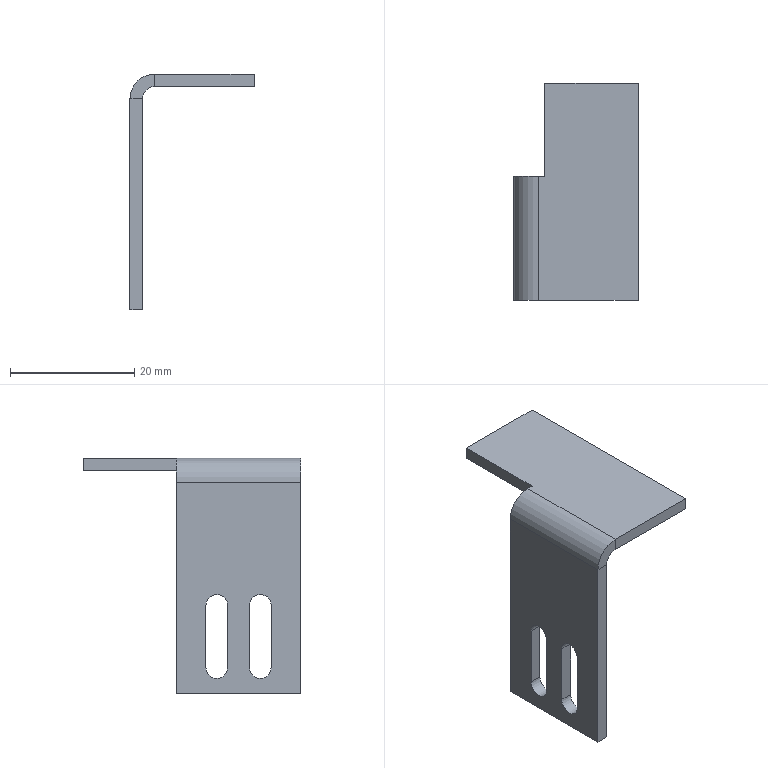Part | STEP file | Slot photoelectric switch sensing plate 1001 | 1 solid | 26 faces | box 20 x 35 x 38 mm | volume 2460 mm3 | plane 18 | cylinder 8 | commonest cylinder face diameters 3.5 x6 4 x1 8 x1